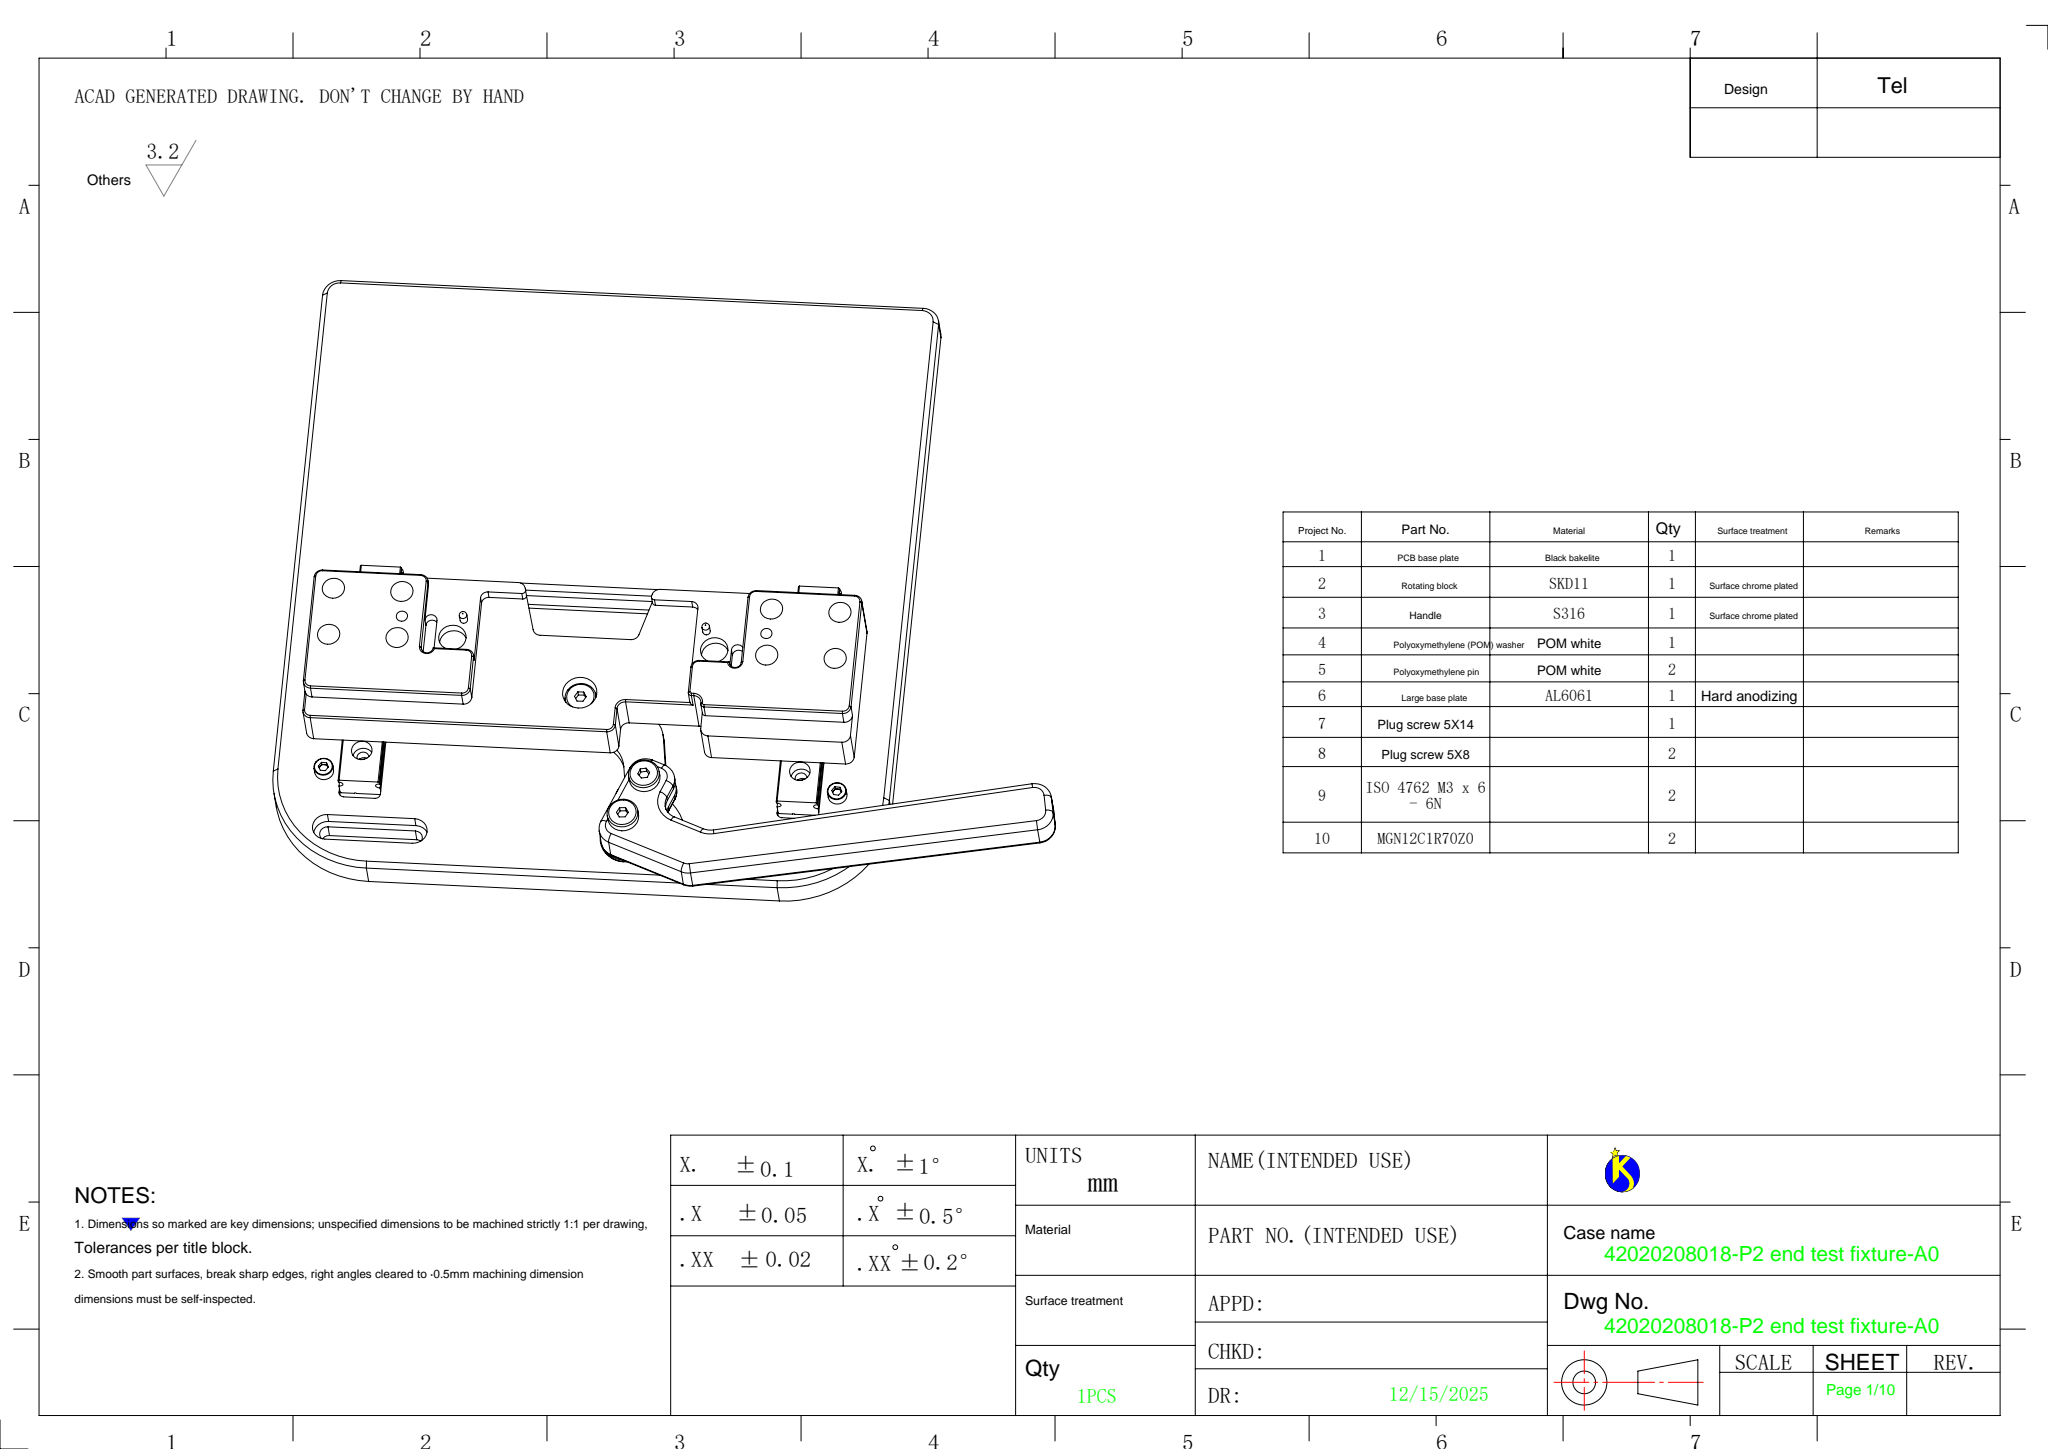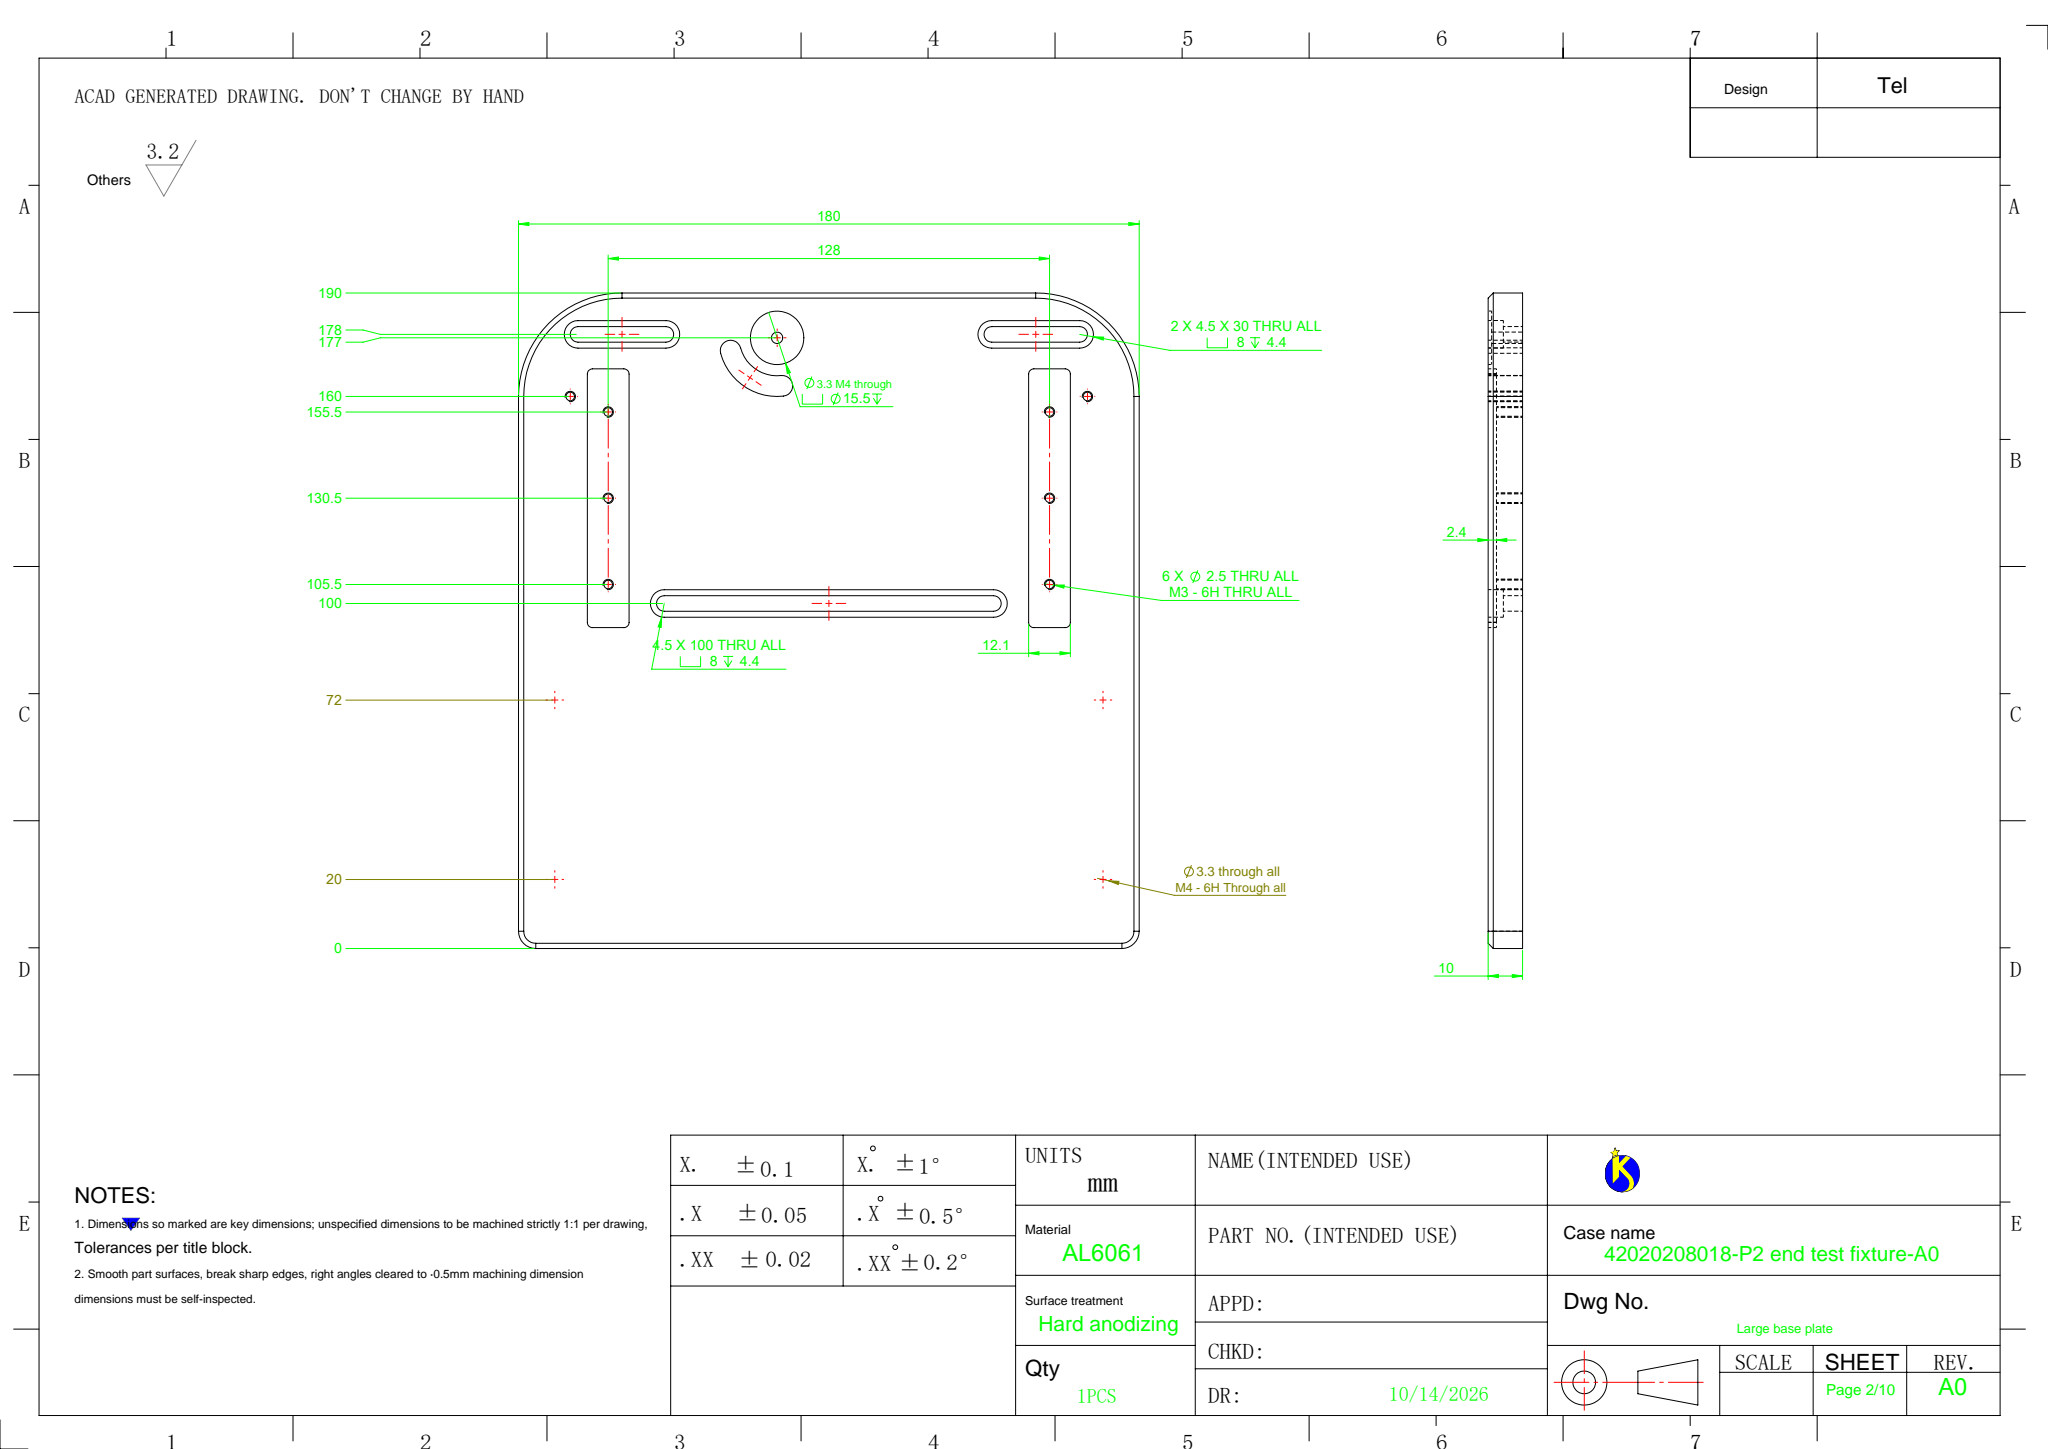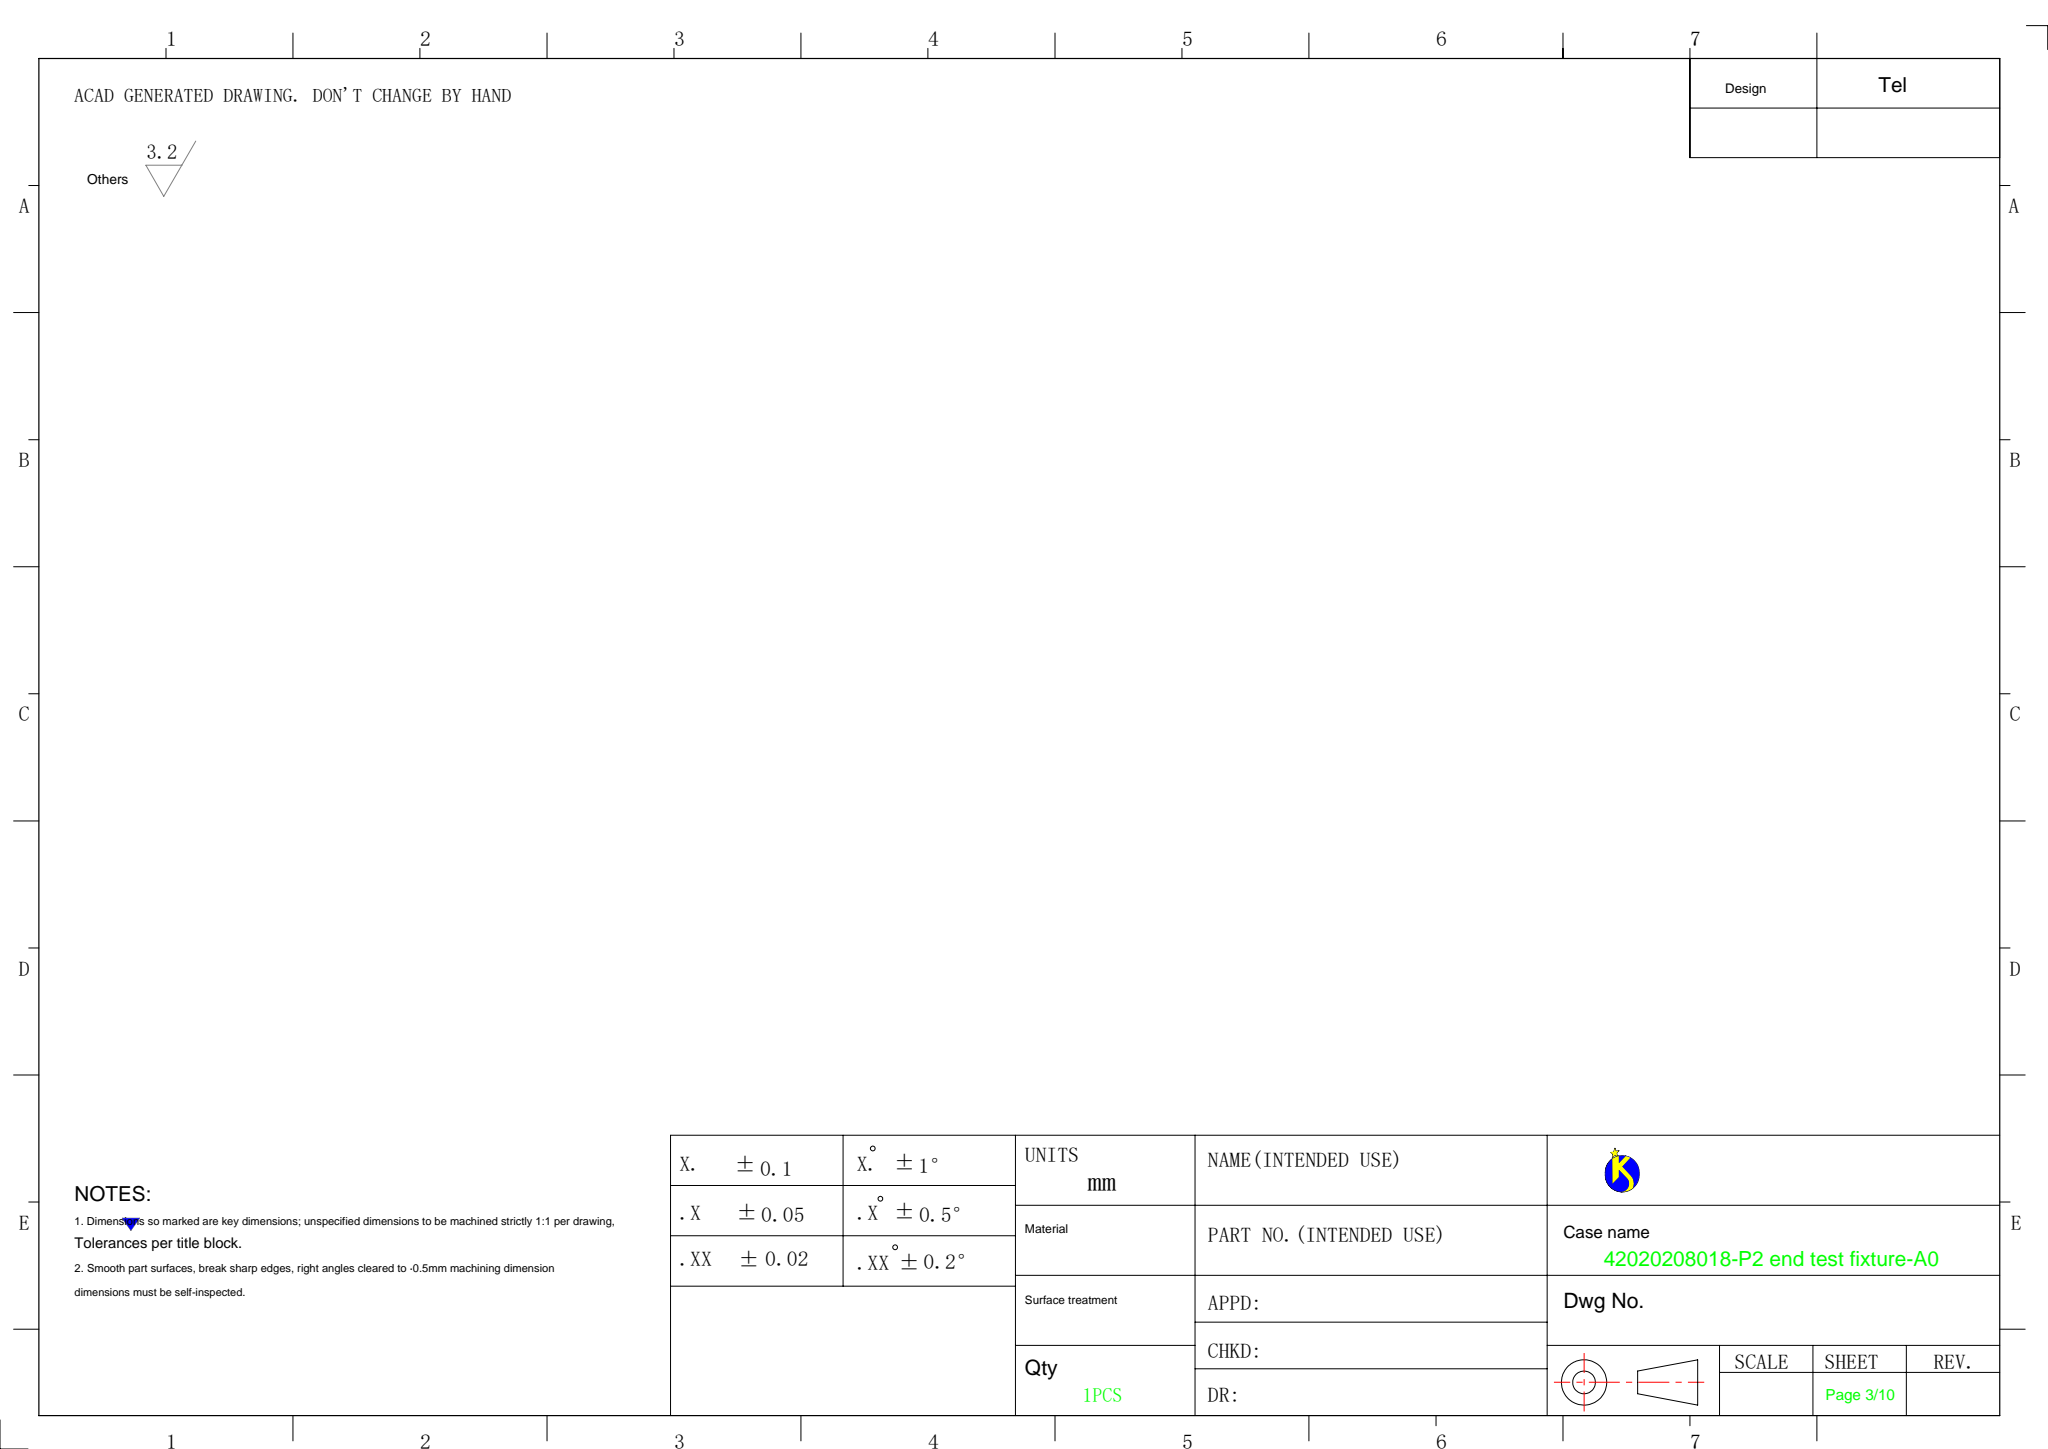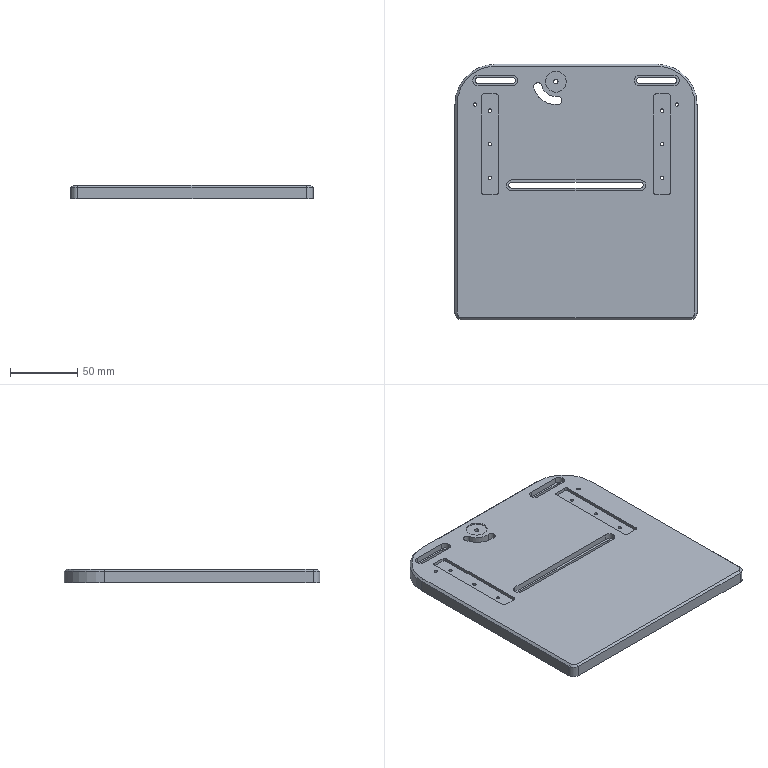Part | SolidWorks | features HoleWzd 4, Attribute 3, Cut 3, Fillet 3, Chamfer 1, Extrusion 1, ICE 1, LPattern 1 | 1 solid | 95 faces | box 180 x 190 x 10 mm | volume 321054 mm3 | cylinder 55 | plane 36 | cone 4 | commonest cylinder face diameters 2.5 x16 4.5 x9 8 x9 3 x8 6 x3 3.3 x2